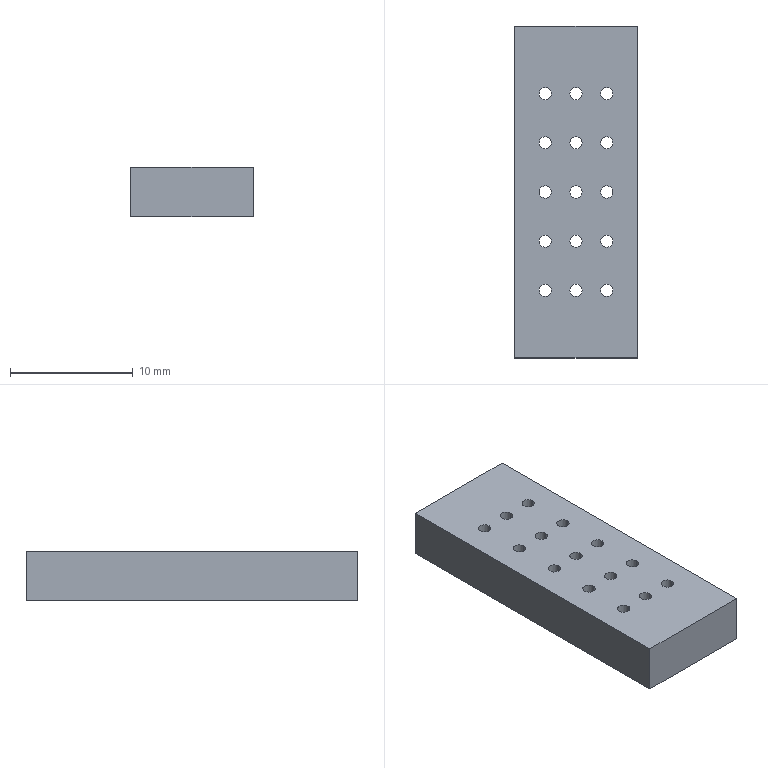Part | SolidWorks | features Extrusion 1, ICE 1, LPattern 1, MirrorPattern 1 | 1 solid | 36 faces | box 10 x 27 x 4 mm | volume 1033 mm3 | cylinder 30 | plane 6 | commonest cylinder face diameters 1 x30
STEP:
#1=CARTESIAN_POINT('',(0.5,4.,0.));
#2=VERTEX_POINT('',#1);
#3=CARTESIAN_POINT('',(-0.5,4.,0.));
#4=VERTEX_POINT('',#3);
#5=CARTESIAN_POINT('',(0.,4.,0.));
#6=DIRECTION('',(0.,0.,-1.));
#7=DIRECTION('',(-1.,0.,0.));
#8=AXIS2_PLACEMENT_3D('',#5,#6,#7);
#9=CIRCLE('',#8,0.5);
#10=EDGE_CURVE('',#2,#4,#9,.T.);
#11=ORIENTED_EDGE('',*,*,#10,.T.);
#12=CARTESIAN_POINT('',(-0.5,4.,4.));
#13=VERTEX_POINT('',#12);
#14=CARTESIAN_POINT('',(-0.5,4.,-0.001));
#15=DIRECTION('',(0.,0.,1.));
#16=VECTOR('',#15,1000.);
#17=LINE('',#14,#16);
#18=EDGE_CURVE('',#4,#13,#17,.T.);
#19=ORIENTED_EDGE('',*,*,#18,.T.);
#20=CARTESIAN_POINT('',(0.5,4.,4.));
#21=VERTEX_POINT('',#20);
#22=CARTESIAN_POINT('',(0.,4.,4.));
#23=DIRECTION('',(0.,0.,-1.));
#24=DIRECTION('',(1.,0.,0.));
#25=AXIS2_PLACEMENT_3D('',#22,#23,#24);
#26=CIRCLE('',#25,0.5);
#27=EDGE_CURVE('',#21,#13,#26,.T.);
#28=ORIENTED_EDGE('',*,*,#27,.F.);
#29=CARTESIAN_POINT('',(0.5,4.,-0.001));
#30=DIRECTION('',(0.,0.,1.));
#31=VECTOR('',#30,1000.);
#32=LINE('',#29,#31);
#33=EDGE_CURVE('',#2,#21,#32,.T.);
#34=ORIENTED_EDGE('',*,*,#33,.F.);
#35=EDGE_LOOP('',(#11,#19,#28,#34));
#36=FACE_OUTER_BOUND('',#35,.T.);
#37=CARTESIAN_POINT('',(0.,4.,-0.001));
#38=DIRECTION('',(0.,0.,1.));
#39=DIRECTION('',(1.,0.,0.));
#40=AXIS2_PLACEMENT_3D('',#37,#38,#39);
#41=CYLINDRICAL_SURFACE('',#40,0.5);
#42=ADVANCED_FACE('',(#36),#41,.F.);
#43=CARTESIAN_POINT('',(-2.,4.,0.));
#44=VERTEX_POINT('',#43);
#45=CARTESIAN_POINT('',(-3.,4.,0.));
#46=VERTEX_POINT('',#45);
#47=CARTESIAN_POINT('',(-2.5,4.,0.));
#48=DIRECTION('',(0.,0.,-1.));
#49=DIRECTION('',(-1.,0.,0.));
#50=AXIS2_PLACEMENT_3D('',#47,#48,#49);
#51=CIRCLE('',#50,0.5);
#52=EDGE_CURVE('',#44,#46,#51,.T.);
#53=ORIENTED_EDGE('',*,*,#52,.T.);
#54=CARTESIAN_POINT('',(-3.,4.,4.));
#55=VERTEX_POINT('',#54);
#56=CARTESIAN_POINT('',(-3.,4.,-0.001));
#57=DIRECTION('',(0.,0.,1.));
#58=VECTOR('',#57,1000.);
#59=LINE('',#56,#58);
#60=EDGE_CURVE('',#46,#55,#59,.T.);
#61=ORIENTED_EDGE('',*,*,#60,.T.);
#62=CARTESIAN_POINT('',(-2.,4.,4.));
#63=VERTEX_POINT('',#62);
#64=CARTESIAN_POINT('',(-2.5,4.,4.));
#65=DIRECTION('',(0.,0.,-1.));
#66=DIRECTION('',(1.,0.,0.));
#67=AXIS2_PLACEMENT_3D('',#64,#65,#66);
#68=CIRCLE('',#67,0.5);
#69=EDGE_CURVE('',#63,#55,#68,.T.);
#70=ORIENTED_EDGE('',*,*,#69,.F.);
#71=CARTESIAN_POINT('',(-2.,4.,-0.001));
#72=DIRECTION('',(0.,0.,1.));
#73=VECTOR('',#72,1000.);
#74=LINE('',#71,#73);
#75=EDGE_CURVE('',#44,#63,#74,.T.);
#76=ORIENTED_EDGE('',*,*,#75,.F.);
#77=EDGE_LOOP('',(#53,#61,#70,#76));
#78=FACE_OUTER_BOUND('',#77,.T.);
#79=CARTESIAN_POINT('',(-2.5,4.,-0.001));
#80=DIRECTION('',(0.,0.,1.));
#81=DIRECTION('',(1.,0.,0.));
#82=AXIS2_PLACEMENT_3D('',#79,#80,#81);
#83=CYLINDRICAL_SURFACE('',#82,0.5);
#84=ADVANCED_FACE('',(#78),#83,.F.);
#85=CARTESIAN_POINT('',(3.,8.,0.));
#86=VERTEX_POINT('',#85);
#87=CARTESIAN_POINT('',(2.,8.,0.));
#88=VERTEX_POINT('',#87);
#89=CARTESIAN_POINT('',(2.5,8.,0.));
#90=DIRECTION('',(0.,0.,-1.));
#91=DIRECTION('',(-1.,0.,0.));
#92=AXIS2_PLACEMENT_3D('',#89,#90,#91);
#93=CIRCLE('',#92,0.5);
#94=EDGE_CURVE('',#86,#88,#93,.T.);
#95=ORIENTED_EDGE('',*,*,#94,.T.);
#96=CARTESIAN_POINT('',(2.,8.,4.));
#97=VERTEX_POINT('',#96);
#98=CARTESIAN_POINT('',(2.,8.,-0.001));
#99=DIRECTION('',(0.,0.,1.));
#100=VECTOR('',#99,1000.);
#101=LINE('',#98,#100);
#102=EDGE_CURVE('',#88,#97,#101,.T.);
#103=ORIENTED_EDGE('',*,*,#102,.T.);
#104=CARTESIAN_POINT('',(3.,8.,4.));
#105=VERTEX_POINT('',#104);
#106=CARTESIAN_POINT('',(2.5,8.,4.));
#107=DIRECTION('',(0.,0.,-1.));
#108=DIRECTION('',(1.,0.,0.));
#109=AXIS2_PLACEMENT_3D('',#106,#107,#108);
#110=CIRCLE('',#109,0.5);
#111=EDGE_CURVE('',#105,#97,#110,.T.);
#112=ORIENTED_EDGE('',*,*,#111,.F.);
#113=CARTESIAN_POINT('',(3.,8.,-0.001));
#114=DIRECTION('',(0.,0.,1.));
#115=VECTOR('',#114,1000.);
#116=LINE('',#113,#115);
#117=EDGE_CURVE('',#86,#105,#116,.T.);
#118=ORIENTED_EDGE('',*,*,#117,.F.);
#119=EDGE_LOOP('',(#95,#103,#112,#118));
#120=FACE_OUTER_BOUND('',#119,.T.);
#121=CARTESIAN_POINT('',(2.5,8.,-0.001));
#122=DIRECTION('',(0.,0.,1.));
#123=DIRECTION('',(1.,0.,0.));
#124=AXIS2_PLACEMENT_3D('',#121,#122,#123);
#125=CYLINDRICAL_SURFACE('',#124,0.5);
#126=ADVANCED_FACE('',(#120),#125,.F.);
#127=CARTESIAN_POINT('',(-2.,8.,0.));
#128=VERTEX_POINT('',#127);
#129=CARTESIAN_POINT('',(-3.,8.,0.));
#130=VERTEX_POINT('',#129);
#131=CARTESIAN_POINT('',(-2.5,8.,0.));
#132=DIRECTION('',(0.,0.,-1.));
#133=DIRECTION('',(-1.,0.,0.));
#134=AXIS2_PLACEMENT_3D('',#131,#132,#133);
#135=CIRCLE('',#134,0.5);
#136=EDGE_CURVE('',#128,#130,#135,.T.);
#137=ORIENTED_EDGE('',*,*,#136,.T.);
#138=CARTESIAN_POINT('',(-3.,8.,4.));
#139=VERTEX_POINT('',#138);
#140=CARTESIAN_POINT('',(-3.,8.,-0.001));
#141=DIRECTION('',(0.,0.,1.));
#142=VECTOR('',#141,1000.);
#143=LINE('',#140,#142);
#144=EDGE_CURVE('',#130,#139,#143,.T.);
#145=ORIENTED_EDGE('',*,*,#144,.T.);
#146=CARTESIAN_POINT('',(-2.,8.,4.));
#147=VERTEX_POINT('',#146);
#148=CARTESIAN_POINT('',(-2.5,8.,4.));
#149=DIRECTION('',(0.,0.,-1.));
#150=DIRECTION('',(1.,0.,0.));
#151=AXIS2_PLACEMENT_3D('',#148,#149,#150);
#152=CIRCLE('',#151,0.5);
#153=EDGE_CURVE('',#147,#139,#152,.T.);
#154=ORIENTED_EDGE('',*,*,#153,.F.);
#155=CARTESIAN_POINT('',(-2.,8.,-0.001));
#156=DIRECTION('',(0.,0.,1.));
#157=VECTOR('',#156,1000.);
#158=LINE('',#155,#157);
#159=EDGE_CURVE('',#128,#147,#158,.T.);
#160=ORIENTED_EDGE('',*,*,#159,.F.);
#161=EDGE_LOOP('',(#137,#145,#154,#160));
#162=FACE_OUTER_BOUND('',#161,.T.);
#163=CARTESIAN_POINT('',(-2.5,8.,-0.001));
#164=DIRECTION('',(0.,0.,1.));
#165=DIRECTION('',(1.,0.,0.));
#166=AXIS2_PLACEMENT_3D('',#163,#164,#165);
#167=CYLINDRICAL_SURFACE('',#166,0.5);
#168=ADVANCED_FACE('',(#162),#167,.F.);
#169=CARTESIAN_POINT('',(0.5,8.,0.));
#170=VERTEX_POINT('',#169);
#171=CARTESIAN_POINT('',(-0.5,8.,0.));
#172=VERTEX_POINT('',#171);
#173=CARTESIAN_POINT('',(0.,8.,0.));
#174=DIRECTION('',(0.,0.,-1.));
#175=DIRECTION('',(-1.,0.,0.));
#176=AXIS2_PLACEMENT_3D('',#173,#174,#175);
#177=CIRCLE('',#176,0.5);
#178=EDGE_CURVE('',#170,#172,#177,.T.);
#179=ORIENTED_EDGE('',*,*,#178,.T.);
#180=CARTESIAN_POINT('',(-0.5,8.,4.));
#181=VERTEX_POINT('',#180);
#182=CARTESIAN_POINT('',(-0.5,8.,-0.001));
#183=DIRECTION('',(0.,0.,1.));
#184=VECTOR('',#183,1000.);
#185=LINE('',#182,#184);
#186=EDGE_CURVE('',#172,#181,#185,.T.);
#187=ORIENTED_EDGE('',*,*,#186,.T.);
#188=CARTESIAN_POINT('',(0.5,8.,4.));
#189=VERTEX_POINT('',#188);
#190=CARTESIAN_POINT('',(0.,8.,4.));
#191=DIRECTION('',(0.,0.,-1.));
#192=DIRECTION('',(1.,0.,0.));
#193=AXIS2_PLACEMENT_3D('',#190,#191,#192);
#194=CIRCLE('',#193,0.5);
#195=EDGE_CURVE('',#189,#181,#194,.T.);
#196=ORIENTED_EDGE('',*,*,#195,.F.);
#197=CARTESIAN_POINT('',(0.5,8.,-0.001));
#198=DIRECTION('',(0.,0.,1.));
#199=VECTOR('',#198,1000.);
#200=LINE('',#197,#199);
#201=EDGE_CURVE('',#170,#189,#200,.T.);
#202=ORIENTED_EDGE('',*,*,#201,.F.);
#203=EDGE_LOOP('',(#179,#187,#196,#202));
#204=FACE_OUTER_BOUND('',#203,.T.);
#205=CARTESIAN_POINT('',(0.,8.,-0.001));
#206=DIRECTION('',(0.,0.,1.));
#207=DIRECTION('',(1.,0.,0.));
#208=AXIS2_PLACEMENT_3D('',#205,#206,#207);
#209=CYLINDRICAL_SURFACE('',#208,0.5);
#210=ADVANCED_FACE('',(#204),#209,.F.);
#211=CARTESIAN_POINT('',(3.,4.,0.));
#212=VERTEX_POINT('',#211);
#213=CARTESIAN_POINT('',(2.,4.,0.));
#214=VERTEX_POINT('',#213);
#215=CARTESIAN_POINT('',(2.5,4.,0.));
#216=DIRECTION('',(0.,0.,-1.));
#217=DIRECTION('',(-1.,0.,0.));
#218=AXIS2_PLACEMENT_3D('',#215,#216,#217);
#219=CIRCLE('',#218,0.5);
#220=EDGE_CURVE('',#212,#214,#219,.T.);
#221=ORIENTED_EDGE('',*,*,#220,.T.);
#222=CARTESIAN_POINT('',(2.,4.,4.));
#223=VERTEX_POINT('',#222);
#224=CARTESIAN_POINT('',(2.,4.,-0.001));
#225=DIRECTION('',(0.,0.,1.));
#226=VECTOR('',#225,1000.);
#227=LINE('',#224,#226);
#228=EDGE_CURVE('',#214,#223,#227,.T.);
#229=ORIENTED_EDGE('',*,*,#228,.T.);
#230=CARTESIAN_POINT('',(3.,4.,4.));
#231=VERTEX_POINT('',#230);
#232=CARTESIAN_POINT('',(2.5,4.,4.));
#233=DIRECTION('',(0.,0.,-1.));
#234=DIRECTION('',(1.,0.,0.));
#235=AXIS2_PLACEMENT_3D('',#232,#233,#234);
#236=CIRCLE('',#235,0.5);
#237=EDGE_CURVE('',#231,#223,#236,.T.);
#238=ORIENTED_EDGE('',*,*,#237,.F.);
#239=CARTESIAN_POINT('',(3.,4.,-0.001));
#240=DIRECTION('',(0.,0.,1.));
#241=VECTOR('',#240,1000.);
#242=LINE('',#239,#241);
#243=EDGE_CURVE('',#212,#231,#242,.T.);
#244=ORIENTED_EDGE('',*,*,#243,.F.);
#245=EDGE_LOOP('',(#221,#229,#238,#244));
#246=FACE_OUTER_BOUND('',#245,.T.);
#247=CARTESIAN_POINT('',(2.5,4.,-0.001));
#248=DIRECTION('',(0.,0.,1.));
#249=DIRECTION('',(1.,0.,0.));
#250=AXIS2_PLACEMENT_3D('',#247,#248,#249);
#251=CYLINDRICAL_SURFACE('',#250,0.5);
#252=ADVANCED_FACE('',(#246),#251,.F.);
#253=CARTESIAN_POINT('',(-3.,-4.,0.));
#254=VERTEX_POINT('',#253);
#255=CARTESIAN_POINT('',(-2.,-4.,0.));
#256=VERTEX_POINT('',#255);
#257=CARTESIAN_POINT('',(-2.5,-4.,0.));
#258=DIRECTION('',(0.,0.,1.));
#259=DIRECTION('',(-1.,0.,0.));
#260=AXIS2_PLACEMENT_3D('',#257,#258,#259);
#261=CIRCLE('',#260,0.5);
#262=EDGE_CURVE('',#254,#256,#261,.T.);
#263=ORIENTED_EDGE('',*,*,#262,.F.);
#264=CARTESIAN_POINT('',(-3.,-4.,4.));
#265=VERTEX_POINT('',#264);
#266=CARTESIAN_POINT('',(-3.,-4.,-0.001));
#267=DIRECTION('',(0.,0.,1.));
#268=VECTOR('',#267,1000.);
#269=LINE('',#266,#268);
#270=EDGE_CURVE('',#254,#265,#269,.T.);
#271=ORIENTED_EDGE('',*,*,#270,.T.);
#272=CARTESIAN_POINT('',(-2.,-4.,4.));
#273=VERTEX_POINT('',#272);
#274=CARTESIAN_POINT('',(-2.5,-4.,4.));
#275=DIRECTION('',(0.,0.,1.));
#276=DIRECTION('',(1.,0.,0.));
#277=AXIS2_PLACEMENT_3D('',#274,#275,#276);
#278=CIRCLE('',#277,0.5);
#279=EDGE_CURVE('',#265,#273,#278,.T.);
#280=ORIENTED_EDGE('',*,*,#279,.T.);
#281=CARTESIAN_POINT('',(-2.,-4.,-0.001));
#282=DIRECTION('',(0.,0.,1.));
#283=VECTOR('',#282,1000.);
#284=LINE('',#281,#283);
#285=EDGE_CURVE('',#256,#273,#284,.T.);
#286=ORIENTED_EDGE('',*,*,#285,.F.);
#287=EDGE_LOOP('',(#263,#271,#280,#286));
#288=FACE_OUTER_BOUND('',#287,.T.);
#289=CARTESIAN_POINT('',(-2.5,-4.,-0.001));
#290=DIRECTION('',(0.,0.,1.));
#291=DIRECTION('',(1.,0.,0.));
#292=AXIS2_PLACEMENT_3D('',#289,#290,#291);
#293=CYLINDRICAL_SURFACE('',#292,0.5);
#294=ADVANCED_FACE('',(#288),#293,.F.);
#295=CARTESIAN_POINT('',(-0.5,-4.,0.));
#296=VERTEX_POINT('',#295);
#297=CARTESIAN_POINT('',(0.5,-4.,0.));
#298=VERTEX_POINT('',#297);
#299=CARTESIAN_POINT('',(0.,-4.,0.));
#300=DIRECTION('',(0.,0.,1.));
#301=DIRECTION('',(-1.,0.,0.));
#302=AXIS2_PLACEMENT_3D('',#299,#300,#301);
#303=CIRCLE('',#302,0.5);
#304=EDGE_CURVE('',#296,#298,#303,.T.);
#305=ORIENTED_EDGE('',*,*,#304,.F.);
#306=CARTESIAN_POINT('',(-0.5,-4.,4.));
#307=VERTEX_POINT('',#306);
#308=CARTESIAN_POINT('',(-0.5,-4.,-0.001));
#309=DIRECTION('',(0.,0.,1.));
#310=VECTOR('',#309,1000.);
#311=LINE('',#308,#310);
#312=EDGE_CURVE('',#296,#307,#311,.T.);
#313=ORIENTED_EDGE('',*,*,#312,.T.);
#314=CARTESIAN_POINT('',(0.5,-4.,4.));
#315=VERTEX_POINT('',#314);
#316=CARTESIAN_POINT('',(0.,-4.,4.));
#317=DIRECTION('',(0.,0.,1.));
#318=DIRECTION('',(1.,0.,0.));
#319=AXIS2_PLACEMENT_3D('',#316,#317,#318);
#320=CIRCLE('',#319,0.5);
#321=EDGE_CURVE('',#307,#315,#320,.T.);
#322=ORIENTED_EDGE('',*,*,#321,.T.);
#323=CARTESIAN_POINT('',(0.5,-4.,-0.001));
#324=DIRECTION('',(0.,0.,1.));
#325=VECTOR('',#324,1000.);
#326=LINE('',#323,#325);
#327=EDGE_CURVE('',#298,#315,#326,.T.);
#328=ORIENTED_EDGE('',*,*,#327,.F.);
#329=EDGE_LOOP('',(#305,#313,#322,#328));
#330=FACE_OUTER_BOUND('',#329,.T.);
#331=CARTESIAN_POINT('',(0.,-4.,-0.001));
#332=DIRECTION('',(0.,0.,1.));
#333=DIRECTION('',(1.,0.,0.));
#334=AXIS2_PLACEMENT_3D('',#331,#332,#333);
#335=CYLINDRICAL_SURFACE('',#334,0.5);
#336=ADVANCED_FACE('',(#330),#335,.F.);
#337=CARTESIAN_POINT('',(2.,-4.,0.));
#338=VERTEX_POINT('',#337);
#339=CARTESIAN_POINT('',(3.,-4.,0.));
#340=VERTEX_POINT('',#339);
#341=CARTESIAN_POINT('',(2.5,-4.,0.));
#342=DIRECTION('',(0.,0.,1.));
#343=DIRECTION('',(-1.,0.,0.));
#344=AXIS2_PLACEMENT_3D('',#341,#342,#343);
#345=CIRCLE('',#344,0.5);
#346=EDGE_CURVE('',#338,#340,#345,.T.);
#347=ORIENTED_EDGE('',*,*,#346,.F.);
#348=CARTESIAN_POINT('',(2.,-4.,4.));
#349=VERTEX_POINT('',#348);
#350=CARTESIAN_POINT('',(2.,-4.,-0.001));
#351=DIRECTION('',(0.,0.,1.));
#352=VECTOR('',#351,1000.);
#353=LINE('',#350,#352);
#354=EDGE_CURVE('',#338,#349,#353,.T.);
#355=ORIENTED_EDGE('',*,*,#354,.T.);
#356=CARTESIAN_POINT('',(3.,-4.,4.));
#357=VERTEX_POINT('',#356);
#358=CARTESIAN_POINT('',(2.5,-4.,4.));
#359=DIRECTION('',(0.,0.,1.));
#360=DIRECTION('',(1.,0.,0.));
#361=AXIS2_PLACEMENT_3D('',#358,#359,#360);
#362=CIRCLE('',#361,0.5);
#363=EDGE_CURVE('',#349,#357,#362,.T.);
#364=ORIENTED_EDGE('',*,*,#363,.T.);
#365=CARTESIAN_POINT('',(3.,-4.,-0.001));
#366=DIRECTION('',(0.,0.,1.));
#367=VECTOR('',#366,1000.);
#368=LINE('',#365,#367);
#369=EDGE_CURVE('',#340,#357,#368,.T.);
#370=ORIENTED_EDGE('',*,*,#369,.F.);
#371=EDGE_LOOP('',(#347,#355,#364,#370));
#372=FACE_OUTER_BOUND('',#371,.T.);
#373=CARTESIAN_POINT('',(2.5,-4.,-0.001));
#374=DIRECTION('',(0.,0.,1.));
#375=DIRECTION('',(1.,0.,0.));
#376=AXIS2_PLACEMENT_3D('',#373,#374,#375);
#377=CYLINDRICAL_SURFACE('',#376,0.5);
#378=ADVANCED_FACE('',(#372),#377,.F.);
#379=CARTESIAN_POINT('',(2.,0.,0.));
#380=VERTEX_POINT('',#379);
#381=CARTESIAN_POINT('',(3.,0.,0.));
#382=VERTEX_POINT('',#381);
#383=CARTESIAN_POINT('',(2.5,0.,0.));
#384=DIRECTION('',(0.,0.,1.));
#385=DIRECTION('',(-1.,0.,0.));
#386=AXIS2_PLACEMENT_3D('',#383,#384,#385);
#387=CIRCLE('',#386,0.5);
#388=EDGE_CURVE('',#380,#382,#387,.T.);
#389=ORIENTED_EDGE('',*,*,#388,.F.);
#390=CARTESIAN_POINT('',(2.,0.,4.));
#391=VERTEX_POINT('',#390);
#392=CARTESIAN_POINT('',(2.,0.,-0.001));
#393=DIRECTION('',(0.,0.,1.));
#394=VECTOR('',#393,1000.);
#395=LINE('',#392,#394);
#396=EDGE_CURVE('',#380,#391,#395,.T.);
#397=ORIENTED_EDGE('',*,*,#396,.T.);
#398=CARTESIAN_POINT('',(3.,0.,4.));
#399=VERTEX_POINT('',#398);
#400=CARTESIAN_POINT('',(2.5,0.,4.));
#401=DIRECTION('',(0.,0.,1.));
#402=DIRECTION('',(1.,0.,0.));
#403=AXIS2_PLACEMENT_3D('',#400,#401,#402);
#404=CIRCLE('',#403,0.5);
#405=EDGE_CURVE('',#391,#399,#404,.T.);
#406=ORIENTED_EDGE('',*,*,#405,.T.);
#407=CARTESIAN_POINT('',(3.,0.,-0.001));
#408=DIRECTION('',(0.,0.,1.));
#409=VECTOR('',#408,1000.);
#410=LINE('',#407,#409);
#411=EDGE_CURVE('',#382,#399,#410,.T.);
#412=ORIENTED_EDGE('',*,*,#411,.F.);
#413=EDGE_LOOP('',(#389,#397,#406,#412));
#414=FACE_OUTER_BOUND('',#413,.T.);
#415=CARTESIAN_POINT('',(2.5,0.,-0.001));
#416=DIRECTION('',(0.,0.,1.));
#417=DIRECTION('',(1.,0.,0.));
#418=AXIS2_PLACEMENT_3D('',#415,#416,#417);
#419=CYLINDRICAL_SURFACE('',#418,0.5);
#420=ADVANCED_FACE('',(#414),#419,.F.);
#421=CARTESIAN_POINT('',(-3.,0.,0.));
#422=VERTEX_POINT('',#421);
#423=CARTESIAN_POINT('',(-2.,0.,0.));
#424=VERTEX_POINT('',#423);
#425=CARTESIAN_POINT('',(-2.5,0.,0.));
#426=DIRECTION('',(0.,0.,1.));
#427=DIRECTION('',(-1.,0.,0.));
#428=AXIS2_PLACEMENT_3D('',#425,#426,#427);
#429=CIRCLE('',#428,0.5);
#430=EDGE_CURVE('',#422,#424,#429,.T.);
#431=ORIENTED_EDGE('',*,*,#430,.F.);
#432=CARTESIAN_POINT('',(-3.,0.,4.));
#433=VERTEX_POINT('',#432);
#434=CARTESIAN_POINT('',(-3.,0.,-0.001));
#435=DIRECTION('',(0.,0.,1.));
#436=VECTOR('',#435,1000.);
#437=LINE('',#434,#436);
#438=EDGE_CURVE('',#422,#433,#437,.T.);
#439=ORIENTED_EDGE('',*,*,#438,.T.);
#440=CARTESIAN_POINT('',(-2.,0.,4.));
#441=VERTEX_POINT('',#440);
#442=CARTESIAN_POINT('',(-2.5,0.,4.));
#443=DIRECTION('',(0.,0.,1.));
#444=DIRECTION('',(1.,0.,0.));
#445=AXIS2_PLACEMENT_3D('',#442,#443,#444);
#446=CIRCLE('',#445,0.5);
#447=EDGE_CURVE('',#433,#441,#446,.T.);
#448=ORIENTED_EDGE('',*,*,#447,.T.);
#449=CARTESIAN_POINT('',(-2.,0.,-0.001));
#450=DIRECTION('',(0.,0.,1.));
#451=VECTOR('',#450,1000.);
#452=LINE('',#449,#451);
#453=EDGE_CURVE('',#424,#441,#452,.T.);
#454=ORIENTED_EDGE('',*,*,#453,.F.);
#455=EDGE_LOOP('',(#431,#439,#448,#454));
#456=FACE_OUTER_BOUND('',#455,.T.);
#457=CARTESIAN_POINT('',(-2.5,0.,-0.001));
#458=DIRECTION('',(0.,0.,1.));
#459=DIRECTION('',(1.,0.,0.));
#460=AXIS2_PLACEMENT_3D('',#457,#458,#459);
#461=CYLINDRICAL_SURFACE('',#460,0.5);
#462=ADVANCED_FACE('',(#456),#461,.F.);
#463=CARTESIAN_POINT('',(-0.5,0.,0.));
#464=VERTEX_POINT('',#463);
#465=CARTESIAN_POINT('',(0.5,0.,0.));
#466=VERTEX_POINT('',#465);
#467=CARTESIAN_POINT('',(0.,0.,0.));
#468=DIRECTION('',(0.,0.,1.));
#469=DIRECTION('',(-1.,0.,0.));
#470=AXIS2_PLACEMENT_3D('',#467,#468,#469);
#471=CIRCLE('',#470,0.5);
#472=EDGE_CURVE('',#464,#466,#471,.T.);
#473=ORIENTED_EDGE('',*,*,#472,.F.);
#474=CARTESIAN_POINT('',(-0.5,0.,4.));
#475=VERTEX_POINT('',#474);
#476=CARTESIAN_POINT('',(-0.5,0.,-0.001));
#477=DIRECTION('',(0.,0.,1.));
#478=VECTOR('',#477,1000.);
#479=LINE('',#476,#478);
#480=EDGE_CURVE('',#464,#475,#479,.T.);
#481=ORIENTED_EDGE('',*,*,#480,.T.);
#482=CARTESIAN_POINT('',(0.5,0.,4.));
#483=VERTEX_POINT('',#482);
#484=CARTESIAN_POINT('',(0.,0.,4.));
#485=DIRECTION('',(0.,0.,1.));
#486=DIRECTION('',(1.,0.,0.));
#487=AXIS2_PLACEMENT_3D('',#484,#485,#486);
#488=CIRCLE('',#487,0.5);
#489=EDGE_CURVE('',#475,#483,#488,.T.);
#490=ORIENTED_EDGE('',*,*,#489,.T.);
#491=CARTESIAN_POINT('',(0.5,0.,-0.001));
#492=DIRECTION('',(0.,0.,1.));
#493=VECTOR('',#492,1000.);
#494=LINE('',#491,#493);
#495=EDGE_CURVE('',#466,#483,#494,.T.);
#496=ORIENTED_EDGE('',*,*,#495,.F.);
#497=EDGE_LOOP('',(#473,#481,#490,#496));
#498=FACE_OUTER_BOUND('',#497,.T.);
#499=CARTESIAN_POINT('',(0.,0.,-0.001));
#500=DIRECTION('',(0.,0.,1.));
#501=DIRECTION('',(1.,0.,0.));
#502=AXIS2_PLACEMENT_3D('',#499,#500,#501);
#503=CYLINDRICAL_SURFACE('',#502,0.5);
#504=ADVANCED_FACE('',(#498),#503,.F.);
#505=CARTESIAN_POINT('',(2.,-8.,0.));
#506=VERTEX_POINT('',#505);
#507=CARTESIAN_POINT('',(3.,-8.,0.));
#508=VERTEX_POINT('',#507);
#509=CARTESIAN_POINT('',(2.5,-8.,0.));
#510=DIRECTION('',(0.,0.,1.));
#511=DIRECTION('',(-1.,0.,0.));
#512=AXIS2_PLACEMENT_3D('',#509,#510,#511);
#513=CIRCLE('',#512,0.5);
#514=EDGE_CURVE('',#506,#508,#513,.T.);
#515=ORIENTED_EDGE('',*,*,#514,.F.);
#516=CARTESIAN_POINT('',(2.,-8.,4.));
#517=VERTEX_POINT('',#516);
#518=CARTESIAN_POINT('',(2.,-8.,-0.001));
#519=DIRECTION('',(0.,0.,1.));
#520=VECTOR('',#519,1000.);
#521=LINE('',#518,#520);
#522=EDGE_CURVE('',#506,#517,#521,.T.);
#523=ORIENTED_EDGE('',*,*,#522,.T.);
#524=CARTESIAN_POINT('',(3.,-8.,4.));
#525=VERTEX_POINT('',#524);
#526=CARTESIAN_POINT('',(2.5,-8.,4.));
#527=DIRECTION('',(0.,0.,1.));
#528=DIRECTION('',(1.,0.,0.));
#529=AXIS2_PLACEMENT_3D('',#526,#527,#528);
#530=CIRCLE('',#529,0.5);
#531=EDGE_CURVE('',#517,#525,#530,.T.);
#532=ORIENTED_EDGE('',*,*,#531,.T.);
#533=CARTESIAN_POINT('',(3.,-8.,-0.001));
#534=DIRECTION('',(0.,0.,1.));
#535=VECTOR('',#534,1000.);
#536=LINE('',#533,#535);
#537=EDGE_CURVE('',#508,#525,#536,.T.);
#538=ORIENTED_EDGE('',*,*,#537,.F.);
#539=EDGE_LOOP('',(#515,#523,#532,#538));
#540=FACE_OUTER_BOUND('',#539,.T.);
#541=CARTESIAN_POINT('',(2.5,-8.,-0.001));
#542=DIRECTION('',(0.,0.,1.));
#543=DIRECTION('',(1.,0.,0.));
#544=AXIS2_PLACEMENT_3D('',#541,#542,#543);
#545=CYLINDRICAL_SURFACE('',#544,0.5);
#546=ADVANCED_FACE('',(#540),#545,.F.);
#547=CARTESIAN_POINT('',(-0.5,-8.,0.));
#548=VERTEX_POINT('',#547);
#549=CARTESIAN_POINT('',(0.5,-8.,0.));
#550=VERTEX_POINT('',#549);
#551=CARTESIAN_POINT('',(0.,-8.,0.));
#552=DIRECTION('',(0.,0.,1.));
#553=DIRECTION('',(-1.,0.,0.));
#554=AXIS2_PLACEMENT_3D('',#551,#552,#553);
#555=CIRCLE('',#554,0.5);
#556=EDGE_CURVE('',#548,#550,#555,.T.);
#557=ORIENTED_EDGE('',*,*,#556,.F.);
#558=CARTESIAN_POINT('',(-0.5,-8.,4.));
#559=VERTEX_POINT('',#558);
#560=CARTESIAN_POINT('',(-0.5,-8.,-0.001));
#561=DIRECTION('',(0.,0.,1.));
#562=VECTOR('',#561,1000.);
#563=LINE('',#560,#562);
#564=EDGE_CURVE('',#548,#559,#563,.T.);
#565=ORIENTED_EDGE('',*,*,#564,.T.);
#566=CARTESIAN_POINT('',(0.5,-8.,4.));
#567=VERTEX_POINT('',#566);
#568=CARTESIAN_POINT('',(0.,-8.,4.));
#569=DIRECTION('',(0.,0.,1.));
#570=DIRECTION('',(1.,0.,0.));
#571=AXIS2_PLACEMENT_3D('',#568,#569,#570);
#572=CIRCLE('',#571,0.5);
#573=EDGE_CURVE('',#559,#567,#572,.T.);
#574=ORIENTED_EDGE('',*,*,#573,.T.);
#575=CARTESIAN_POINT('',(0.5,-8.,-0.001));
#576=DIRECTION('',(0.,0.,1.));
#577=VECTOR('',#576,1000.);
#578=LINE('',#575,#577);
#579=EDGE_CURVE('',#550,#567,#578,.T.);
#580=ORIENTED_EDGE('',*,*,#579,.F.);
#581=EDGE_LOOP('',(#557,#565,#574,#580));
#582=FACE_OUTER_BOUND('',#581,.T.);
#583=CARTESIAN_POINT('',(0.,-8.,-0.001));
#584=DIRECTION('',(0.,0.,1.));
#585=DIRECTION('',(1.,0.,0.));
#586=AXIS2_PLACEMENT_3D('',#583,#584,#585);
#587=CYLINDRICAL_SURFACE('',#586,0.5);
#588=ADVANCED_FACE('',(#582),#587,.F.);
#589=CARTESIAN_POINT('',(-3.,-8.,0.));
#590=VERTEX_POINT('',#589);
#591=CARTESIAN_POINT('',(-2.,-8.,0.));
#592=VERTEX_POINT('',#591);
#593=CARTESIAN_POINT('',(-2.5,-8.,0.));
#594=DIRECTION('',(0.,0.,1.));
#595=DIRECTION('',(-1.,0.,0.));
#596=AXIS2_PLACEMENT_3D('',#593,#594,#595);
#597=CIRCLE('',#596,0.5);
#598=EDGE_CURVE('',#590,#592,#597,.T.);
#599=ORIENTED_EDGE('',*,*,#598,.F.);
#600=CARTESIAN_POINT('',(-3.,-8.,4.));
#601=VERTEX_POINT('',#600);
#602=CARTESIAN_POINT('',(-3.,-8.,-0.001));
#603=DIRECTION('',(0.,0.,1.));
#604=VECTOR('',#603,1000.);
#605=LINE('',#602,#604);
#606=EDGE_CURVE('',#590,#601,#605,.T.);
#607=ORIENTED_EDGE('',*,*,#606,.T.);
#608=CARTESIAN_POINT('',(-2.,-8.,4.));
#609=VERTEX_POINT('',#608);
#610=CARTESIAN_POINT('',(-2.5,-8.,4.));
#611=DIRECTION('',(0.,0.,1.));
#612=DIRECTION('',(1.,0.,0.));
#613=AXIS2_PLACEMENT_3D('',#610,#611,#612);
#614=CIRCLE('',#613,0.5);
#615=EDGE_CURVE('',#601,#609,#614,.T.);
#616=ORIENTED_EDGE('',*,*,#615,.T.);
#617=CARTESIAN_POINT('',(-2.,-8.,-0.001));
#618=DIRECTION('',(0.,0.,1.));
#619=VECTOR('',#618,1000.);
#620=LINE('',#617,#619);
#621=EDGE_CURVE('',#592,#609,#620,.T.);
#622=ORIENTED_EDGE('',*,*,#621,.F.);
#623=EDGE_LOOP('',(#599,#607,#616,#622));
#624=FACE_OUTER_BOUND('',#623,.T.);
#625=CARTESIAN_POINT('',(-2.5,-8.,-0.001));
#626=DIRECTION('',(0.,0.,1.));
#627=DIRECTION('',(1.,0.,0.));
#628=AXIS2_PLACEMENT_3D('',#625,#626,#627);
#629=CYLINDRICAL_SURFACE('',#628,0.5);
#630=ADVANCED_FACE('',(#624),#629,.F.);
#631=CARTESIAN_POINT('',(-2.5,-4.,4.));
#632=DIRECTION('',(0.,0.,1.));
#633=DIRECTION('',(1.,0.,0.));
#634=AXIS2_PLACEMENT_3D('',#631,#632,#633);
#635=CIRCLE('',#634,0.5);
#636=EDGE_CURVE('',#273,#265,#635,.T.);
#637=ORIENTED_EDGE('',*,*,#636,.F.);
#638=ORIENTED_EDGE('',*,*,#279,.F.);
#639=EDGE_LOOP('',(#637,#638));
#640=FACE_BOUND('',#639,.T.);
#641=CARTESIAN_POINT('',(0.,-4.,4.));
#642=DIRECTION('',(0.,0.,1.));
#643=DIRECTION('',(1.,0.,0.));
#644=AXIS2_PLACEMENT_3D('',#641,#642,#643);
#645=CIRCLE('',#644,0.5);
#646=EDGE_CURVE('',#315,#307,#645,.T.);
#647=ORIENTED_EDGE('',*,*,#646,.F.);
#648=ORIENTED_EDGE('',*,*,#321,.F.);
#649=EDGE_LOOP('',(#647,#648));
#650=FACE_BOUND('',#649,.T.);
#651=CARTESIAN_POINT('',(2.5,-4.,4.));
#652=DIRECTION('',(0.,0.,1.));
#653=DIRECTION('',(1.,0.,0.));
#654=AXIS2_PLACEMENT_3D('',#651,#652,#653);
#655=CIRCLE('',#654,0.5);
#656=EDGE_CURVE('',#357,#349,#655,.T.);
#657=ORIENTED_EDGE('',*,*,#656,.F.);
#658=ORIENTED_EDGE('',*,*,#363,.F.);
#659=EDGE_LOOP('',(#657,#658));
#660=FACE_BOUND('',#659,.T.);
#661=CARTESIAN_POINT('',(2.5,0.,4.));
#662=DIRECTION('',(0.,0.,1.));
#663=DIRECTION('',(1.,0.,0.));
#664=AXIS2_PLACEMENT_3D('',#661,#662,#663);
#665=CIRCLE('',#664,0.5);
#666=EDGE_CURVE('',#399,#391,#665,.T.);
#667=ORIENTED_EDGE('',*,*,#666,.F.);
#668=ORIENTED_EDGE('',*,*,#405,.F.);
#669=EDGE_LOOP('',(#667,#668));
#670=FACE_BOUND('',#669,.T.);
#671=CARTESIAN_POINT('',(-2.5,0.,4.));
#672=DIRECTION('',(0.,0.,1.));
#673=DIRECTION('',(1.,0.,0.));
#674=AXIS2_PLACEMENT_3D('',#671,#672,#673);
#675=CIRCLE('',#674,0.5);
#676=EDGE_CURVE('',#441,#433,#675,.T.);
#677=ORIENTED_EDGE('',*,*,#676,.F.);
#678=ORIENTED_EDGE('',*,*,#447,.F.);
#679=EDGE_LOOP('',(#677,#678));
#680=FACE_BOUND('',#679,.T.);
#681=CARTESIAN_POINT('',(0.,0.,4.));
#682=DIRECTION('',(0.,0.,1.));
#683=DIRECTION('',(1.,0.,0.));
#684=AXIS2_PLACEMENT_3D('',#681,#682,#683);
#685=CIRCLE('',#684,0.5);
#686=EDGE_CURVE('',#483,#475,#685,.T.);
#687=ORIENTED_EDGE('',*,*,#686,.F.);
#688=ORIENTED_EDGE('',*,*,#489,.F.);
#689=EDGE_LOOP('',(#687,#688));
#690=FACE_BOUND('',#689,.T.);
#691=CARTESIAN_POINT('',(5.,-13.5,4.));
#692=VERTEX_POINT('',#691);
#693=CARTESIAN_POINT('',(5.,13.5,4.));
#694=VERTEX_POINT('',#693);
#695=CARTESIAN_POINT('',(5.,-13.5,4.));
#696=DIRECTION('',(0.,1.,0.));
#697=VECTOR('',#696,1000.);
#698=LINE('',#695,#697);
#699=EDGE_CURVE('',#692,#694,#698,.T.);
#700=ORIENTED_EDGE('',*,*,#699,.T.);
#701=CARTESIAN_POINT('',(-5.,13.5,4.));
#702=VERTEX_POINT('',#701);
#703=CARTESIAN_POINT('',(-5.,13.5,4.));
#704=DIRECTION('',(-1.,0.,0.));
#705=VECTOR('',#704,1000.);
#706=LINE('',#703,#705);
#707=EDGE_CURVE('',#694,#702,#706,.T.);
#708=ORIENTED_EDGE('',*,*,#707,.T.);
#709=CARTESIAN_POINT('',(-5.,-13.5,4.));
#710=VERTEX_POINT('',#709);
#711=CARTESIAN_POINT('',(-5.,-13.5,4.));
#712=DIRECTION('',(0.,-1.,0.));
#713=VECTOR('',#712,1000.);
#714=LINE('',#711,#713);
#715=EDGE_CURVE('',#702,#710,#714,.T.);
#716=ORIENTED_EDGE('',*,*,#715,.T.);
#717=CARTESIAN_POINT('',(-5.,-13.5,4.));
#718=DIRECTION('',(1.,0.,0.));
#719=VECTOR('',#718,1000.);
#720=LINE('',#717,#719);
#721=EDGE_CURVE('',#710,#692,#720,.T.);
#722=ORIENTED_EDGE('',*,*,#721,.T.);
#723=EDGE_LOOP('',(#700,#708,#716,#722));
#724=FACE_OUTER_BOUND('',#723,.T.);
#725=CARTESIAN_POINT('',(2.5,-8.,4.));
#726=DIRECTION('',(0.,0.,1.));
#727=DIRECTION('',(1.,0.,0.));
#728=AXIS2_PLACEMENT_3D('',#725,#726,#727);
#729=CIRCLE('',#728,0.5);
#730=EDGE_CURVE('',#525,#517,#729,.T.);
#731=ORIENTED_EDGE('',*,*,#730,.F.);
#732=ORIENTED_EDGE('',*,*,#531,.F.);
#733=EDGE_LOOP('',(#731,#732));
#734=FACE_BOUND('',#733,.T.);
#735=CARTESIAN_POINT('',(0.,-8.,4.));
#736=DIRECTION('',(0.,0.,1.));
#737=DIRECTION('',(1.,0.,0.));
#738=AXIS2_PLACEMENT_3D('',#735,#736,#737);
#739=CIRCLE('',#738,0.5);
#740=EDGE_CURVE('',#567,#559,#739,.T.);
#741=ORIENTED_EDGE('',*,*,#740,.F.);
#742=ORIENTED_EDGE('',*,*,#573,.F.);
#743=EDGE_LOOP('',(#741,#742));
#744=FACE_BOUND('',#743,.T.);
#745=CARTESIAN_POINT('',(-2.5,-8.,4.));
#746=DIRECTION('',(0.,0.,1.));
#747=DIRECTION('',(1.,0.,0.));
#748=AXIS2_PLACEMENT_3D('',#745,#746,#747);
#749=CIRCLE('',#748,0.5);
#750=EDGE_CURVE('',#609,#601,#749,.T.);
#751=ORIENTED_EDGE('',*,*,#750,.F.);
#752=ORIENTED_EDGE('',*,*,#615,.F.);
#753=EDGE_LOOP('',(#751,#752));
#754=FACE_BOUND('',#753,.T.);
#755=ORIENTED_EDGE('',*,*,#237,.T.);
#756=CARTESIAN_POINT('',(2.5,4.,4.));
#757=DIRECTION('',(0.,0.,-1.));
#758=DIRECTION('',(1.,0.,0.));
#759=AXIS2_PLACEMENT_3D('',#756,#757,#758);
#760=CIRCLE('',#759,0.5);
#761=EDGE_CURVE('',#223,#231,#760,.T.);
#762=ORIENTED_EDGE('',*,*,#761,.T.);
#763=EDGE_LOOP('',(#755,#762));
#764=FACE_BOUND('',#763,.T.);
#765=ORIENTED_EDGE('',*,*,#195,.T.);
#766=CARTESIAN_POINT('',(0.,8.,4.));
#767=DIRECTION('',(0.,0.,-1.));
#768=DIRECTION('',(1.,0.,0.));
#769=AXIS2_PLACEMENT_3D('',#766,#767,#768);
#770=CIRCLE('',#769,0.5);
#771=EDGE_CURVE('',#181,#189,#770,.T.);
#772=ORIENTED_EDGE('',*,*,#771,.T.);
#773=EDGE_LOOP('',(#765,#772));
#774=FACE_BOUND('',#773,.T.);
#775=ORIENTED_EDGE('',*,*,#153,.T.);
#776=CARTESIAN_POINT('',(-2.5,8.,4.));
#777=DIRECTION('',(0.,0.,-1.));
#778=DIRECTION('',(1.,0.,0.));
#779=AXIS2_PLACEMENT_3D('',#776,#777,#778);
#780=CIRCLE('',#779,0.5);
#781=EDGE_CURVE('',#139,#147,#780,.T.);
#782=ORIENTED_EDGE('',*,*,#781,.T.);
#783=EDGE_LOOP('',(#775,#782));
#784=FACE_BOUND('',#783,.T.);
#785=ORIENTED_EDGE('',*,*,#111,.T.);
#786=CARTESIAN_POINT('',(2.5,8.,4.));
#787=DIRECTION('',(0.,0.,-1.));
#788=DIRECTION('',(1.,0.,0.));
#789=AXIS2_PLACEMENT_3D('',#786,#787,#788);
#790=CIRCLE('',#789,0.5);
#791=EDGE_CURVE('',#97,#105,#790,.T.);
#792=ORIENTED_EDGE('',*,*,#791,.T.);
#793=EDGE_LOOP('',(#785,#792));
#794=FACE_BOUND('',#793,.T.);
#795=ORIENTED_EDGE('',*,*,#69,.T.);
#796=CARTESIAN_POINT('',(-2.5,4.,4.));
#797=DIRECTION('',(0.,0.,-1.));
#798=DIRECTION('',(1.,0.,0.));
#799=AXIS2_PLACEMENT_3D('',#796,#797,#798);
#800=CIRCLE('',#799,0.5);
#801=EDGE_CURVE('',#55,#63,#800,.T.);
#802=ORIENTED_EDGE('',*,*,#801,.T.);
#803=EDGE_LOOP('',(#795,#802));
#804=FACE_BOUND('',#803,.T.);
#805=ORIENTED_EDGE('',*,*,#27,.T.);
#806=CARTESIAN_POINT('',(0.,4.,4.));
#807=DIRECTION('',(0.,0.,-1.));
#808=DIRECTION('',(1.,0.,0.));
#809=AXIS2_PLACEMENT_3D('',#806,#807,#808);
#810=CIRCLE('',#809,0.5);
#811=EDGE_CURVE('',#13,#21,#810,.T.);
#812=ORIENTED_EDGE('',*,*,#811,.T.);
#813=EDGE_LOOP('',(#805,#812));
#814=FACE_BOUND('',#813,.T.);
#815=CARTESIAN_POINT('',(0.,0.,4.));
#816=DIRECTION('',(0.,0.,-1.));
#817=DIRECTION('',(-1.,0.,0.));
#818=AXIS2_PLACEMENT_3D('',#815,#816,#817);
#819=PLANE('',#818);
#820=ADVANCED_FACE('',(#640,#650,#660,#670,#680,#690,#724,#734,#744,#754,#764,#774,#784,#794,#804,#814),#819,.F.);
#821=ORIENTED_EDGE('',*,*,#52,.F.);
#822=CARTESIAN_POINT('',(-2.5,4.,0.));
#823=DIRECTION('',(0.,0.,-1.));
#824=DIRECTION('',(-1.,0.,0.));
#825=AXIS2_PLACEMENT_3D('',#822,#823,#824);
#826=CIRCLE('',#825,0.5);
#827=EDGE_CURVE('',#46,#44,#826,.T.);
#828=ORIENTED_EDGE('',*,*,#827,.F.);
#829=EDGE_LOOP('',(#821,#828));
#830=FACE_BOUND('',#829,.T.);
#831=ORIENTED_EDGE('',*,*,#136,.F.);
#832=CARTESIAN_POINT('',(-2.5,8.,0.));
#833=DIRECTION('',(0.,0.,-1.));
#834=DIRECTION('',(-1.,0.,0.));
#835=AXIS2_PLACEMENT_3D('',#832,#833,#834);
#836=CIRCLE('',#835,0.5);
#837=EDGE_CURVE('',#130,#128,#836,.T.);
#838=ORIENTED_EDGE('',*,*,#837,.F.);
#839=EDGE_LOOP('',(#831,#838));
#840=FACE_BOUND('',#839,.T.);
#841=ORIENTED_EDGE('',*,*,#220,.F.);
#842=CARTESIAN_POINT('',(2.5,4.,0.));
#843=DIRECTION('',(0.,0.,-1.));
#844=DIRECTION('',(-1.,0.,0.));
#845=AXIS2_PLACEMENT_3D('',#842,#843,#844);
#846=CIRCLE('',#845,0.5);
#847=EDGE_CURVE('',#214,#212,#846,.T.);
#848=ORIENTED_EDGE('',*,*,#847,.F.);
#849=EDGE_LOOP('',(#841,#848));
#850=FACE_BOUND('',#849,.T.);
#851=CARTESIAN_POINT('',(-2.5,-4.,0.));
#852=DIRECTION('',(0.,0.,1.));
#853=DIRECTION('',(-1.,0.,0.));
#854=AXIS2_PLACEMENT_3D('',#851,#852,#853);
#855=CIRCLE('',#854,0.5);
#856=EDGE_CURVE('',#256,#254,#855,.T.);
#857=ORIENTED_EDGE('',*,*,#856,.T.);
#858=ORIENTED_EDGE('',*,*,#262,.T.);
#859=EDGE_LOOP('',(#857,#858));
#860=FACE_BOUND('',#859,.T.);
#861=CARTESIAN_POINT('',(0.,-4.,0.));
#862=DIRECTION('',(0.,0.,1.));
#863=DIRECTION('',(-1.,0.,0.));
#864=AXIS2_PLACEMENT_3D('',#861,#862,#863);
#865=CIRCLE('',#864,0.5);
#866=EDGE_CURVE('',#298,#296,#865,.T.);
#867=ORIENTED_EDGE('',*,*,#866,.T.);
#868=ORIENTED_EDGE('',*,*,#304,.T.);
#869=EDGE_LOOP('',(#867,#868));
#870=FACE_BOUND('',#869,.T.);
#871=CARTESIAN_POINT('',(2.5,-4.,0.));
#872=DIRECTION('',(0.,0.,1.));
#873=DIRECTION('',(-1.,0.,0.));
#874=AXIS2_PLACEMENT_3D('',#871,#872,#873);
#875=CIRCLE('',#874,0.5);
#876=EDGE_CURVE('',#340,#338,#875,.T.);
#877=ORIENTED_EDGE('',*,*,#876,.T.);
#878=ORIENTED_EDGE('',*,*,#346,.T.);
#879=EDGE_LOOP('',(#877,#878));
#880=FACE_BOUND('',#879,.T.);
#881=CARTESIAN_POINT('',(2.5,0.,0.));
#882=DIRECTION('',(0.,0.,1.));
#883=DIRECTION('',(-1.,0.,0.));
#884=AXIS2_PLACEMENT_3D('',#881,#882,#883);
#885=CIRCLE('',#884,0.5);
#886=EDGE_CURVE('',#382,#380,#885,.T.);
#887=ORIENTED_EDGE('',*,*,#886,.T.);
#888=ORIENTED_EDGE('',*,*,#388,.T.);
#889=EDGE_LOOP('',(#887,#888));
#890=FACE_BOUND('',#889,.T.);
#891=CARTESIAN_POINT('',(-2.5,0.,0.));
#892=DIRECTION('',(0.,0.,1.));
#893=DIRECTION('',(-1.,0.,0.));
#894=AXIS2_PLACEMENT_3D('',#891,#892,#893);
#895=CIRCLE('',#894,0.5);
#896=EDGE_CURVE('',#424,#422,#895,.T.);
#897=ORIENTED_EDGE('',*,*,#896,.T.);
#898=ORIENTED_EDGE('',*,*,#430,.T.);
#899=EDGE_LOOP('',(#897,#898));
#900=FACE_BOUND('',#899,.T.);
#901=CARTESIAN_POINT('',(0.,0.,0.));
#902=DIRECTION('',(0.,0.,1.));
#903=DIRECTION('',(-1.,0.,0.));
#904=AXIS2_PLACEMENT_3D('',#901,#902,#903);
#905=CIRCLE('',#904,0.5);
#906=EDGE_CURVE('',#466,#464,#905,.T.);
#907=ORIENTED_EDGE('',*,*,#906,.T.);
#908=ORIENTED_EDGE('',*,*,#472,.T.);
#909=EDGE_LOOP('',(#907,#908));
#910=FACE_BOUND('',#909,.T.);
#911=CARTESIAN_POINT('',(5.,-13.5,0.));
#912=VERTEX_POINT('',#911);
#913=CARTESIAN_POINT('',(5.,13.5,0.));
#914=VERTEX_POINT('',#913);
#915=CARTESIAN_POINT('',(5.,-13.5,0.));
#916=DIRECTION('',(0.,1.,0.));
#917=VECTOR('',#916,1000.);
#918=LINE('',#915,#917);
#919=EDGE_CURVE('',#912,#914,#918,.T.);
#920=ORIENTED_EDGE('',*,*,#919,.F.);
#921=CARTESIAN_POINT('',(-5.,-13.5,0.));
#922=VERTEX_POINT('',#921);
#923=CARTESIAN_POINT('',(-5.,-13.5,0.));
#924=DIRECTION('',(1.,0.,0.));
#925=VECTOR('',#924,1000.);
#926=LINE('',#923,#925);
#927=EDGE_CURVE('',#922,#912,#926,.T.);
#928=ORIENTED_EDGE('',*,*,#927,.F.);
#929=CARTESIAN_POINT('',(-5.,13.5,0.));
#930=VERTEX_POINT('',#929);
#931=CARTESIAN_POINT('',(-5.,-13.5,0.));
#932=DIRECTION('',(0.,-1.,0.));
#933=VECTOR('',#932,1000.);
#934=LINE('',#931,#933);
#935=EDGE_CURVE('',#930,#922,#934,.T.);
#936=ORIENTED_EDGE('',*,*,#935,.F.);
#937=CARTESIAN_POINT('',(-5.,13.5,0.));
#938=DIRECTION('',(-1.,0.,0.));
#939=VECTOR('',#938,1000.);
#940=LINE('',#937,#939);
#941=EDGE_CURVE('',#914,#930,#940,.T.);
#942=ORIENTED_EDGE('',*,*,#941,.F.);
#943=EDGE_LOOP('',(#920,#928,#936,#942));
#944=FACE_OUTER_BOUND('',#943,.T.);
#945=CARTESIAN_POINT('',(2.5,-8.,0.));
#946=DIRECTION('',(0.,0.,1.));
#947=DIRECTION('',(-1.,0.,0.));
#948=AXIS2_PLACEMENT_3D('',#945,#946,#947);
#949=CIRCLE('',#948,0.5);
#950=EDGE_CURVE('',#508,#506,#949,.T.);
#951=ORIENTED_EDGE('',*,*,#950,.T.);
#952=ORIENTED_EDGE('',*,*,#514,.T.);
#953=EDGE_LOOP('',(#951,#952));
#954=FACE_BOUND('',#953,.T.);
#955=CARTESIAN_POINT('',(0.,-8.,0.));
#956=DIRECTION('',(0.,0.,1.));
#957=DIRECTION('',(-1.,0.,0.));
#958=AXIS2_PLACEMENT_3D('',#955,#956,#957);
#959=CIRCLE('',#958,0.5);
#960=EDGE_CURVE('',#550,#548,#959,.T.);
#961=ORIENTED_EDGE('',*,*,#960,.T.);
#962=ORIENTED_EDGE('',*,*,#556,.T.);
#963=EDGE_LOOP('',(#961,#962));
#964=FACE_BOUND('',#963,.T.);
#965=CARTESIAN_POINT('',(-2.5,-8.,0.));
#966=DIRECTION('',(0.,0.,1.));
#967=DIRECTION('',(-1.,0.,0.));
#968=AXIS2_PLACEMENT_3D('',#965,#966,#967);
#969=CIRCLE('',#968,0.5);
#970=EDGE_CURVE('',#592,#590,#969,.T.);
#971=ORIENTED_EDGE('',*,*,#970,.T.);
#972=ORIENTED_EDGE('',*,*,#598,.T.);
#973=EDGE_LOOP('',(#971,#972));
#974=FACE_BOUND('',#973,.T.);
#975=ORIENTED_EDGE('',*,*,#178,.F.);
#976=CARTESIAN_POINT('',(0.,8.,0.));
#977=DIRECTION('',(0.,0.,-1.));
#978=DIRECTION('',(-1.,0.,0.));
#979=AXIS2_PLACEMENT_3D('',#976,#977,#978);
#980=CIRCLE('',#979,0.5);
#981=EDGE_CURVE('',#172,#170,#980,.T.);
#982=ORIENTED_EDGE('',*,*,#981,.F.);
#983=EDGE_LOOP('',(#975,#982));
#984=FACE_BOUND('',#983,.T.);
#985=ORIENTED_EDGE('',*,*,#94,.F.);
#986=CARTESIAN_POINT('',(2.5,8.,0.));
#987=DIRECTION('',(0.,0.,-1.));
#988=DIRECTION('',(-1.,0.,0.));
#989=AXIS2_PLACEMENT_3D('',#986,#987,#988);
#990=CIRCLE('',#989,0.5);
#991=EDGE_CURVE('',#88,#86,#990,.T.);
#992=ORIENTED_EDGE('',*,*,#991,.F.);
#993=EDGE_LOOP('',(#985,#992));
#994=FACE_BOUND('',#993,.T.);
#995=ORIENTED_EDGE('',*,*,#10,.F.);
#996=CARTESIAN_POINT('',(0.,4.,0.));
#997=DIRECTION('',(0.,0.,-1.));
#998=DIRECTION('',(-1.,0.,0.));
#999=AXIS2_PLACEMENT_3D('',#996,#997,#998);
#1000=CIRCLE('',#999,0.5);
#1001=EDGE_CURVE('',#4,#2,#1000,.T.);
#1002=ORIENTED_EDGE('',*,*,#1001,.F.);
#1003=EDGE_LOOP('',(#995,#1002));
#1004=FACE_BOUND('',#1003,.T.);
#1005=CARTESIAN_POINT('',(0.,0.,0.));
#1006=DIRECTION('',(0.,0.,-1.));
#1007=DIRECTION('',(-1.,0.,0.));
#1008=AXIS2_PLACEMENT_3D('',#1005,#1006,#1007);
#1009=PLANE('',#1008);
#1010=ADVANCED_FACE('',(#830,#840,#850,#860,#870,#880,#890,#900,#910,#944,#954,#964,#974,#984,#994,#1004),#1009,.T.);
#1011=ORIENTED_EDGE('',*,*,#606,.F.);
#1012=ORIENTED_EDGE('',*,*,#970,.F.);
#1013=ORIENTED_EDGE('',*,*,#621,.T.);
#1014=ORIENTED_EDGE('',*,*,#750,.T.);
#1015=EDGE_LOOP('',(#1011,#1012,#1013,#1014));
#1016=FACE_OUTER_BOUND('',#1015,.T.);
#1017=CARTESIAN_POINT('',(-2.5,-8.,-0.001));
#1018=DIRECTION('',(0.,0.,1.));
#1019=DIRECTION('',(1.,0.,0.));
#1020=AXIS2_PLACEMENT_3D('',#1017,#1018,#1019);
#1021=CYLINDRICAL_SURFACE('',#1020,0.5);
#1022=ADVANCED_FACE('',(#1016),#1021,.F.);
#1023=ORIENTED_EDGE('',*,*,#564,.F.);
#1024=ORIENTED_EDGE('',*,*,#960,.F.);
#1025=ORIENTED_EDGE('',*,*,#579,.T.);
#1026=ORIENTED_EDGE('',*,*,#740,.T.);
#1027=EDGE_LOOP('',(#1023,#1024,#1025,#1026));
#1028=FACE_OUTER_BOUND('',#1027,.T.);
#1029=CARTESIAN_POINT('',(0.,-8.,-0.001));
#1030=DIRECTION('',(0.,0.,1.));
#1031=DIRECTION('',(1.,0.,0.));
#1032=AXIS2_PLACEMENT_3D('',#1029,#1030,#1031);
#1033=CYLINDRICAL_SURFACE('',#1032,0.5);
#1034=ADVANCED_FACE('',(#1028),#1033,.F.);
#1035=ORIENTED_EDGE('',*,*,#522,.F.);
#1036=ORIENTED_EDGE('',*,*,#950,.F.);
#1037=ORIENTED_EDGE('',*,*,#537,.T.);
#1038=ORIENTED_EDGE('',*,*,#730,.T.);
#1039=EDGE_LOOP('',(#1035,#1036,#1037,#1038));
#1040=FACE_OUTER_BOUND('',#1039,.T.);
#1041=CARTESIAN_POINT('',(2.5,-8.,-0.001));
#1042=DIRECTION('',(0.,0.,1.));
#1043=DIRECTION('',(1.,0.,0.));
#1044=AXIS2_PLACEMENT_3D('',#1041,#1042,#1043);
#1045=CYLINDRICAL_SURFACE('',#1044,0.5);
#1046=ADVANCED_FACE('',(#1040),#1045,.F.);
#1047=ORIENTED_EDGE('',*,*,#919,.T.);
#1048=CARTESIAN_POINT('',(5.,13.5,4.));
#1049=DIRECTION('',(0.,0.,-1.));
#1050=VECTOR('',#1049,1000.);
#1051=LINE('',#1048,#1050);
#1052=EDGE_CURVE('',#694,#914,#1051,.T.);
#1053=ORIENTED_EDGE('',*,*,#1052,.F.);
#1054=ORIENTED_EDGE('',*,*,#699,.F.);
#1055=CARTESIAN_POINT('',(5.,-13.5,4.));
#1056=DIRECTION('',(0.,0.,-1.));
#1057=VECTOR('',#1056,1000.);
#1058=LINE('',#1055,#1057);
#1059=EDGE_CURVE('',#692,#912,#1058,.T.);
#1060=ORIENTED_EDGE('',*,*,#1059,.T.);
#1061=EDGE_LOOP('',(#1047,#1053,#1054,#1060));
#1062=FACE_OUTER_BOUND('',#1061,.T.);
#1063=CARTESIAN_POINT('',(5.,-13.5,4.));
#1064=DIRECTION('',(-1.,0.,0.));
#1065=DIRECTION('',(0.,0.,1.));
#1066=AXIS2_PLACEMENT_3D('',#1063,#1064,#1065);
#1067=PLANE('',#1066);
#1068=ADVANCED_FACE('',(#1062),#1067,.F.);
#1069=ORIENTED_EDGE('',*,*,#941,.T.);
#1070=CARTESIAN_POINT('',(-5.,13.5,4.));
#1071=DIRECTION('',(0.,0.,-1.));
#1072=VECTOR('',#1071,1000.);
#1073=LINE('',#1070,#1072);
#1074=EDGE_CURVE('',#702,#930,#1073,.T.);
#1075=ORIENTED_EDGE('',*,*,#1074,.F.);
#1076=ORIENTED_EDGE('',*,*,#707,.F.);
#1077=ORIENTED_EDGE('',*,*,#1052,.T.);
#1078=EDGE_LOOP('',(#1069,#1075,#1076,#1077));
#1079=FACE_OUTER_BOUND('',#1078,.T.);
#1080=CARTESIAN_POINT('',(-5.,13.5,4.));
#1081=DIRECTION('',(0.,-1.,0.));
#1082=DIRECTION('',(0.,0.,-1.));
#1083=AXIS2_PLACEMENT_3D('',#1080,#1081,#1082);
#1084=PLANE('',#1083);
#1085=ADVANCED_FACE('',(#1079),#1084,.F.);
#1086=ORIENTED_EDGE('',*,*,#935,.T.);
#1087=CARTESIAN_POINT('',(-5.,-13.5,4.));
#1088=DIRECTION('',(0.,0.,-1.));
#1089=VECTOR('',#1088,1000.);
#1090=LINE('',#1087,#1089);
#1091=EDGE_CURVE('',#710,#922,#1090,.T.);
#1092=ORIENTED_EDGE('',*,*,#1091,.F.);
#1093=ORIENTED_EDGE('',*,*,#715,.F.);
#1094=ORIENTED_EDGE('',*,*,#1074,.T.);
#1095=EDGE_LOOP('',(#1086,#1092,#1093,#1094));
#1096=FACE_OUTER_BOUND('',#1095,.T.);
#1097=CARTESIAN_POINT('',(-5.,-13.5,4.));
#1098=DIRECTION('',(1.,0.,0.));
#1099=DIRECTION('',(0.,0.,-1.));
#1100=AXIS2_PLACEMENT_3D('',#1097,#1098,#1099);
#1101=PLANE('',#1100);
#1102=ADVANCED_FACE('',(#1096),#1101,.F.);
#1103=ORIENTED_EDGE('',*,*,#927,.T.);
#1104=ORIENTED_EDGE('',*,*,#1059,.F.);
#1105=ORIENTED_EDGE('',*,*,#721,.F.);
#1106=ORIENTED_EDGE('',*,*,#1091,.T.);
#1107=EDGE_LOOP('',(#1103,#1104,#1105,#1106));
#1108=FACE_OUTER_BOUND('',#1107,.T.);
#1109=CARTESIAN_POINT('',(-5.,-13.5,4.));
#1110=DIRECTION('',(0.,1.,0.));
#1111=DIRECTION('',(0.,0.,1.));
#1112=AXIS2_PLACEMENT_3D('',#1109,#1110,#1111);
#1113=PLANE('',#1112);
#1114=ADVANCED_FACE('',(#1108),#1113,.F.);
#1115=ORIENTED_EDGE('',*,*,#480,.F.);
#1116=ORIENTED_EDGE('',*,*,#906,.F.);
#1117=ORIENTED_EDGE('',*,*,#495,.T.);
#1118=ORIENTED_EDGE('',*,*,#686,.T.);
#1119=EDGE_LOOP('',(#1115,#1116,#1117,#1118));
#1120=FACE_OUTER_BOUND('',#1119,.T.);
#1121=CARTESIAN_POINT('',(0.,0.,-0.001));
#1122=DIRECTION('',(0.,0.,1.));
#1123=DIRECTION('',(1.,0.,0.));
#1124=AXIS2_PLACEMENT_3D('',#1121,#1122,#1123);
#1125=CYLINDRICAL_SURFACE('',#1124,0.5);
#1126=ADVANCED_FACE('',(#1120),#1125,.F.);
#1127=ORIENTED_EDGE('',*,*,#438,.F.);
#1128=ORIENTED_EDGE('',*,*,#896,.F.);
#1129=ORIENTED_EDGE('',*,*,#453,.T.);
#1130=ORIENTED_EDGE('',*,*,#676,.T.);
#1131=EDGE_LOOP('',(#1127,#1128,#1129,#1130));
#1132=FACE_OUTER_BOUND('',#1131,.T.);
#1133=CARTESIAN_POINT('',(-2.5,0.,-0.001));
#1134=DIRECTION('',(0.,0.,1.));
#1135=DIRECTION('',(1.,0.,0.));
#1136=AXIS2_PLACEMENT_3D('',#1133,#1134,#1135);
#1137=CYLINDRICAL_SURFACE('',#1136,0.5);
#1138=ADVANCED_FACE('',(#1132),#1137,.F.);
#1139=ORIENTED_EDGE('',*,*,#396,.F.);
#1140=ORIENTED_EDGE('',*,*,#886,.F.);
#1141=ORIENTED_EDGE('',*,*,#411,.T.);
#1142=ORIENTED_EDGE('',*,*,#666,.T.);
#1143=EDGE_LOOP('',(#1139,#1140,#1141,#1142));
#1144=FACE_OUTER_BOUND('',#1143,.T.);
#1145=CARTESIAN_POINT('',(2.5,0.,-0.001));
#1146=DIRECTION('',(0.,0.,1.));
#1147=DIRECTION('',(1.,0.,0.));
#1148=AXIS2_PLACEMENT_3D('',#1145,#1146,#1147);
#1149=CYLINDRICAL_SURFACE('',#1148,0.5);
#1150=ADVANCED_FACE('',(#1144),#1149,.F.);
#1151=ORIENTED_EDGE('',*,*,#354,.F.);
#1152=ORIENTED_EDGE('',*,*,#876,.F.);
#1153=ORIENTED_EDGE('',*,*,#369,.T.);
#1154=ORIENTED_EDGE('',*,*,#656,.T.);
#1155=EDGE_LOOP('',(#1151,#1152,#1153,#1154));
#1156=FACE_OUTER_BOUND('',#1155,.T.);
#1157=CARTESIAN_POINT('',(2.5,-4.,-0.001));
#1158=DIRECTION('',(0.,0.,1.));
#1159=DIRECTION('',(1.,0.,0.));
#1160=AXIS2_PLACEMENT_3D('',#1157,#1158,#1159);
#1161=CYLINDRICAL_SURFACE('',#1160,0.5);
#1162=ADVANCED_FACE('',(#1156),#1161,.F.);
#1163=ORIENTED_EDGE('',*,*,#312,.F.);
#1164=ORIENTED_EDGE('',*,*,#866,.F.);
#1165=ORIENTED_EDGE('',*,*,#327,.T.);
#1166=ORIENTED_EDGE('',*,*,#646,.T.);
#1167=EDGE_LOOP('',(#1163,#1164,#1165,#1166));
#1168=FACE_OUTER_BOUND('',#1167,.T.);
#1169=CARTESIAN_POINT('',(0.,-4.,-0.001));
#1170=DIRECTION('',(0.,0.,1.));
#1171=DIRECTION('',(1.,0.,0.));
#1172=AXIS2_PLACEMENT_3D('',#1169,#1170,#1171);
#1173=CYLINDRICAL_SURFACE('',#1172,0.5);
#1174=ADVANCED_FACE('',(#1168),#1173,.F.);
#1175=ORIENTED_EDGE('',*,*,#270,.F.);
#1176=ORIENTED_EDGE('',*,*,#856,.F.);
#1177=ORIENTED_EDGE('',*,*,#285,.T.);
#1178=ORIENTED_EDGE('',*,*,#636,.T.);
#1179=EDGE_LOOP('',(#1175,#1176,#1177,#1178));
#1180=FACE_OUTER_BOUND('',#1179,.T.);
#1181=CARTESIAN_POINT('',(-2.5,-4.,-0.001));
#1182=DIRECTION('',(0.,0.,1.));
#1183=DIRECTION('',(1.,0.,0.));
#1184=AXIS2_PLACEMENT_3D('',#1181,#1182,#1183);
#1185=CYLINDRICAL_SURFACE('',#1184,0.5);
#1186=ADVANCED_FACE('',(#1180),#1185,.F.);
#1187=ORIENTED_EDGE('',*,*,#228,.F.);
#1188=ORIENTED_EDGE('',*,*,#847,.T.);
#1189=ORIENTED_EDGE('',*,*,#243,.T.);
#1190=ORIENTED_EDGE('',*,*,#761,.F.);
#1191=EDGE_LOOP('',(#1187,#1188,#1189,#1190));
#1192=FACE_OUTER_BOUND('',#1191,.T.);
#1193=CARTESIAN_POINT('',(2.5,4.,-0.001));
#1194=DIRECTION('',(0.,0.,1.));
#1195=DIRECTION('',(1.,0.,0.));
#1196=AXIS2_PLACEMENT_3D('',#1193,#1194,#1195);
#1197=CYLINDRICAL_SURFACE('',#1196,0.5);
#1198=ADVANCED_FACE('',(#1192),#1197,.F.);
#1199=ORIENTED_EDGE('',*,*,#186,.F.);
#1200=ORIENTED_EDGE('',*,*,#981,.T.);
#1201=ORIENTED_EDGE('',*,*,#201,.T.);
#1202=ORIENTED_EDGE('',*,*,#771,.F.);
#1203=EDGE_LOOP('',(#1199,#1200,#1201,#1202));
#1204=FACE_OUTER_BOUND('',#1203,.T.);
#1205=CARTESIAN_POINT('',(0.,8.,-0.001));
#1206=DIRECTION('',(0.,0.,1.));
#1207=DIRECTION('',(1.,0.,0.));
#1208=AXIS2_PLACEMENT_3D('',#1205,#1206,#1207);
#1209=CYLINDRICAL_SURFACE('',#1208,0.5);
#1210=ADVANCED_FACE('',(#1204),#1209,.F.);
#1211=ORIENTED_EDGE('',*,*,#144,.F.);
#1212=ORIENTED_EDGE('',*,*,#837,.T.);
#1213=ORIENTED_EDGE('',*,*,#159,.T.);
#1214=ORIENTED_EDGE('',*,*,#781,.F.);
#1215=EDGE_LOOP('',(#1211,#1212,#1213,#1214));
#1216=FACE_OUTER_BOUND('',#1215,.T.);
#1217=CARTESIAN_POINT('',(-2.5,8.,-0.001));
#1218=DIRECTION('',(0.,0.,1.));
#1219=DIRECTION('',(1.,0.,0.));
#1220=AXIS2_PLACEMENT_3D('',#1217,#1218,#1219);
#1221=CYLINDRICAL_SURFACE('',#1220,0.5);
#1222=ADVANCED_FACE('',(#1216),#1221,.F.);
#1223=ORIENTED_EDGE('',*,*,#102,.F.);
#1224=ORIENTED_EDGE('',*,*,#991,.T.);
#1225=ORIENTED_EDGE('',*,*,#117,.T.);
#1226=ORIENTED_EDGE('',*,*,#791,.F.);
#1227=EDGE_LOOP('',(#1223,#1224,#1225,#1226));
#1228=FACE_OUTER_BOUND('',#1227,.T.);
#1229=CARTESIAN_POINT('',(2.5,8.,-0.001));
#1230=DIRECTION('',(0.,0.,1.));
#1231=DIRECTION('',(1.,0.,0.));
#1232=AXIS2_PLACEMENT_3D('',#1229,#1230,#1231);
#1233=CYLINDRICAL_SURFACE('',#1232,0.5);
#1234=ADVANCED_FACE('',(#1228),#1233,.F.);
#1235=ORIENTED_EDGE('',*,*,#60,.F.);
#1236=ORIENTED_EDGE('',*,*,#827,.T.);
#1237=ORIENTED_EDGE('',*,*,#75,.T.);
#1238=ORIENTED_EDGE('',*,*,#801,.F.);
#1239=EDGE_LOOP('',(#1235,#1236,#1237,#1238));
#1240=FACE_OUTER_BOUND('',#1239,.T.);
#1241=CARTESIAN_POINT('',(-2.5,4.,-0.001));
#1242=DIRECTION('',(0.,0.,1.));
#1243=DIRECTION('',(1.,0.,0.));
#1244=AXIS2_PLACEMENT_3D('',#1241,#1242,#1243);
#1245=CYLINDRICAL_SURFACE('',#1244,0.5);
#1246=ADVANCED_FACE('',(#1240),#1245,.F.);
#1247=ORIENTED_EDGE('',*,*,#18,.F.);
#1248=ORIENTED_EDGE('',*,*,#1001,.T.);
#1249=ORIENTED_EDGE('',*,*,#33,.T.);
#1250=ORIENTED_EDGE('',*,*,#811,.F.);
#1251=EDGE_LOOP('',(#1247,#1248,#1249,#1250));
#1252=FACE_OUTER_BOUND('',#1251,.T.);
#1253=CARTESIAN_POINT('',(0.,4.,-0.001));
#1254=DIRECTION('',(0.,0.,1.));
#1255=DIRECTION('',(1.,0.,0.));
#1256=AXIS2_PLACEMENT_3D('',#1253,#1254,#1255);
#1257=CYLINDRICAL_SURFACE('',#1256,0.5);
#1258=ADVANCED_FACE('',(#1252),#1257,.F.);
#1259=CLOSED_SHELL('',(#42,#84,#126,#168,#210,#252,#294,#336,#378,#420,#462,#504,#546,#588,#630,#820,#1010,#1022,#1034,#1046,#1068,#1085,#1102,#1114,#1126,#1138,#1150,#1162,#1174,#1186,#1198,#1210,#1222,#1234,#1246,#1258));
#1260=MANIFOLD_SOLID_BREP('',#1259);
#1261=CARTESIAN_POINT('',(0.,0.,0.));
#1262=DIRECTION('',(0.,0.,1.));
#1263=DIRECTION('',(1.,0.,0.));
#1264=AXIS2_PLACEMENT_3D('',#1261,#1262,#1263);
#1265=(LENGTH_UNIT()NAMED_UNIT(*)SI_UNIT(.MILLI.,.METRE.));
#1266=UNCERTAINTY_MEASURE_WITH_UNIT(LENGTH_MEASURE(0.00001),#1265,'','');
#1267=(NAMED_UNIT(*)PLANE_ANGLE_UNIT()SI_UNIT($,.RADIAN.));
#1268=(NAMED_UNIT(*)SI_UNIT($,.STERADIAN.)SOLID_ANGLE_UNIT());
#1269=(GEOMETRIC_REPRESENTATION_CONTEXT(3)GLOBAL_UNCERTAINTY_ASSIGNED_CONTEXT((#1266))GLOBAL_UNIT_ASSIGNED_CONTEXT((#1265,#1267,#1268))REPRESENTATION_CONTEXT('',''));
#1270=ADVANCED_BREP_SHAPE_REPRESENTATION('',(#1260,#1264),#1269);